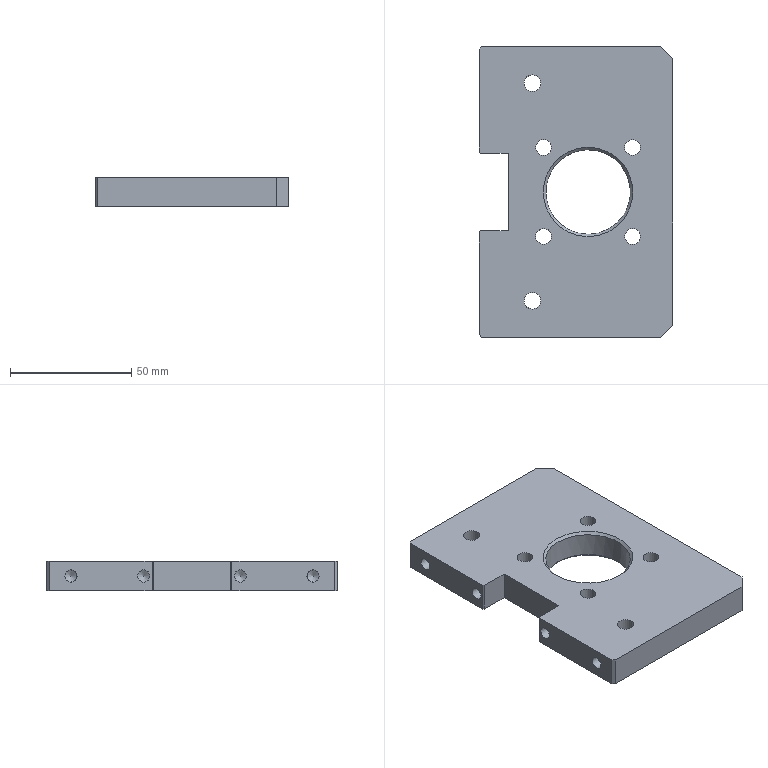Part | NX | 1 solid | 33 faces | box 80 x 120 x 12 mm | volume 94547 mm3 | plane 16 | cylinder 11 | cone 6 | commonest cylinder face diameters 5 x4 6.5 x4 6.8 x2 35 x1
STEP:
#1=CARTESIAN_POINT('',(-18.,41.6,0.));
#2=VERTEX_POINT('',#1);
#3=CARTESIAN_POINT('',(-18.,45.,0.));
#4=DIRECTION('',(0.,0.,1.));
#5=DIRECTION('',(0.,-1.,0.));
#6=AXIS2_PLACEMENT_3D('',#3,#4,#5);
#7=CIRCLE('',#6,3.4);
#8=EDGE_CURVE('',#2,#2,#7,.T.);
#9=ORIENTED_EDGE('',*,*,#8,.F.);
#10=EDGE_LOOP('',(#9));
#11=FACE_BOUND('',#10,.T.);
#12=CARTESIAN_POINT('',(5.,18.5,0.));
#13=VERTEX_POINT('',#12);
#14=CARTESIAN_POINT('',(5.,0.,0.));
#15=DIRECTION('',(0.,0.,-1.));
#16=DIRECTION('',(0.,1.,0.));
#17=AXIS2_PLACEMENT_3D('',#14,#15,#16);
#18=CIRCLE('',#17,18.5);
#19=EDGE_CURVE('',#13,#13,#18,.T.);
#20=ORIENTED_EDGE('',*,*,#19,.T.);
#21=EDGE_LOOP('',(#20));
#22=FACE_BOUND('',#21,.T.);
#23=CARTESIAN_POINT('',(23.385,-15.135,0.));
#24=VERTEX_POINT('',#23);
#25=CARTESIAN_POINT('',(23.385,-18.385,0.));
#26=DIRECTION('',(0.,0.,1.));
#27=DIRECTION('',(0.,1.,0.));
#28=AXIS2_PLACEMENT_3D('',#25,#26,#27);
#29=CIRCLE('',#28,3.25);
#30=EDGE_CURVE('',#24,#24,#29,.T.);
#31=ORIENTED_EDGE('',*,*,#30,.F.);
#32=EDGE_LOOP('',(#31));
#33=FACE_BOUND('',#32,.T.);
#34=CARTESIAN_POINT('',(-10.135,-18.385,0.));
#35=VERTEX_POINT('',#34);
#36=CARTESIAN_POINT('',(-13.385,-18.385,0.));
#37=DIRECTION('',(0.,0.,1.));
#38=DIRECTION('',(1.,0.,0.));
#39=AXIS2_PLACEMENT_3D('',#36,#37,#38);
#40=CIRCLE('',#39,3.25);
#41=EDGE_CURVE('',#35,#35,#40,.T.);
#42=ORIENTED_EDGE('',*,*,#41,.F.);
#43=EDGE_LOOP('',(#42));
#44=FACE_BOUND('',#43,.T.);
#45=CARTESIAN_POINT('',(-13.385,15.135,0.));
#46=VERTEX_POINT('',#45);
#47=CARTESIAN_POINT('',(-13.385,18.385,0.));
#48=DIRECTION('',(0.,0.,1.));
#49=DIRECTION('',(0.,-1.,0.));
#50=AXIS2_PLACEMENT_3D('',#47,#48,#49);
#51=CIRCLE('',#50,3.25);
#52=EDGE_CURVE('',#46,#46,#51,.T.);
#53=ORIENTED_EDGE('',*,*,#52,.F.);
#54=EDGE_LOOP('',(#53));
#55=FACE_BOUND('',#54,.T.);
#56=CARTESIAN_POINT('',(20.135,18.385,0.));
#57=VERTEX_POINT('',#56);
#58=CARTESIAN_POINT('',(23.385,18.385,0.));
#59=DIRECTION('',(0.,0.,1.));
#60=DIRECTION('',(-1.,0.,0.));
#61=AXIS2_PLACEMENT_3D('',#58,#59,#60);
#62=CIRCLE('',#61,3.25);
#63=EDGE_CURVE('',#57,#57,#62,.T.);
#64=ORIENTED_EDGE('',*,*,#63,.F.);
#65=EDGE_LOOP('',(#64));
#66=FACE_BOUND('',#65,.T.);
#67=CARTESIAN_POINT('',(-39.5,-16.,0.));
#68=VERTEX_POINT('',#67);
#69=CARTESIAN_POINT('',(-28.,-16.,0.));
#70=VERTEX_POINT('',#69);
#71=CARTESIAN_POINT('',(-52.,-16.,0.));
#72=DIRECTION('',(1.,0.,0.));
#73=VECTOR('',#72,1000.);
#74=LINE('',#71,#73);
#75=EDGE_CURVE('',#68,#70,#74,.T.);
#76=ORIENTED_EDGE('',*,*,#75,.F.);
#77=CARTESIAN_POINT('',(-40.,-16.5,0.));
#78=VERTEX_POINT('',#77);
#79=CARTESIAN_POINT('',(-40.,-16.5,0.));
#80=DIRECTION('',(0.7071,0.7071,0.));
#81=VECTOR('',#80,1000.);
#82=LINE('',#79,#81);
#83=EDGE_CURVE('',#68,#78,#82,.F.);
#84=ORIENTED_EDGE('',*,*,#83,.T.);
#85=CARTESIAN_POINT('',(-40.,-59.,0.));
#86=VERTEX_POINT('',#85);
#87=CARTESIAN_POINT('',(-40.,-60.,0.));
#88=DIRECTION('',(0.,1.,0.));
#89=VECTOR('',#88,1000.);
#90=LINE('',#87,#89);
#91=EDGE_CURVE('',#86,#78,#90,.T.);
#92=ORIENTED_EDGE('',*,*,#91,.F.);
#93=CARTESIAN_POINT('',(-39.,-60.,0.));
#94=VERTEX_POINT('',#93);
#95=CARTESIAN_POINT('',(-39.,-60.,0.));
#96=DIRECTION('',(-0.7071,0.7071,0.));
#97=VECTOR('',#96,1000.);
#98=LINE('',#95,#97);
#99=EDGE_CURVE('',#86,#94,#98,.F.);
#100=ORIENTED_EDGE('',*,*,#99,.T.);
#101=CARTESIAN_POINT('',(35.,-60.,0.));
#102=VERTEX_POINT('',#101);
#103=CARTESIAN_POINT('',(-40.,-60.,0.));
#104=DIRECTION('',(-1.,0.,0.));
#105=VECTOR('',#104,1000.);
#106=LINE('',#103,#105);
#107=EDGE_CURVE('',#102,#94,#106,.T.);
#108=ORIENTED_EDGE('',*,*,#107,.F.);
#109=CARTESIAN_POINT('',(40.,-55.,0.));
#110=VERTEX_POINT('',#109);
#111=CARTESIAN_POINT('',(40.,-55.,0.));
#112=DIRECTION('',(-0.7071,-0.7071,0.));
#113=VECTOR('',#112,1000.);
#114=LINE('',#111,#113);
#115=EDGE_CURVE('',#110,#102,#114,.T.);
#116=ORIENTED_EDGE('',*,*,#115,.F.);
#117=CARTESIAN_POINT('',(40.,55.,0.));
#118=VERTEX_POINT('',#117);
#119=CARTESIAN_POINT('',(40.,-60.,0.));
#120=DIRECTION('',(0.,1.,0.));
#121=VECTOR('',#120,1000.);
#122=LINE('',#119,#121);
#123=EDGE_CURVE('',#110,#118,#122,.T.);
#124=ORIENTED_EDGE('',*,*,#123,.T.);
#125=CARTESIAN_POINT('',(35.,60.,0.));
#126=VERTEX_POINT('',#125);
#127=CARTESIAN_POINT('',(40.,55.,0.));
#128=DIRECTION('',(0.7071,-0.7071,0.));
#129=VECTOR('',#128,1000.);
#130=LINE('',#127,#129);
#131=EDGE_CURVE('',#126,#118,#130,.T.);
#132=ORIENTED_EDGE('',*,*,#131,.F.);
#133=CARTESIAN_POINT('',(-39.,60.,0.));
#134=VERTEX_POINT('',#133);
#135=CARTESIAN_POINT('',(-40.,60.,0.));
#136=DIRECTION('',(-1.,0.,0.));
#137=VECTOR('',#136,1000.);
#138=LINE('',#135,#137);
#139=EDGE_CURVE('',#126,#134,#138,.T.);
#140=ORIENTED_EDGE('',*,*,#139,.T.);
#141=CARTESIAN_POINT('',(-40.,59.,0.));
#142=VERTEX_POINT('',#141);
#143=CARTESIAN_POINT('',(-40.,59.,0.));
#144=DIRECTION('',(-0.7071,-0.7071,0.));
#145=VECTOR('',#144,1000.);
#146=LINE('',#143,#145);
#147=EDGE_CURVE('',#134,#142,#146,.T.);
#148=ORIENTED_EDGE('',*,*,#147,.T.);
#149=CARTESIAN_POINT('',(-40.,16.5,0.));
#150=VERTEX_POINT('',#149);
#151=CARTESIAN_POINT('',(-40.,-60.,0.));
#152=DIRECTION('',(0.,1.,0.));
#153=VECTOR('',#152,1000.);
#154=LINE('',#151,#153);
#155=EDGE_CURVE('',#150,#142,#154,.T.);
#156=ORIENTED_EDGE('',*,*,#155,.F.);
#157=CARTESIAN_POINT('',(-39.5,16.,0.));
#158=VERTEX_POINT('',#157);
#159=CARTESIAN_POINT('',(-40.,16.5,0.));
#160=DIRECTION('',(-0.7071,0.7071,0.));
#161=VECTOR('',#160,1000.);
#162=LINE('',#159,#161);
#163=EDGE_CURVE('',#150,#158,#162,.F.);
#164=ORIENTED_EDGE('',*,*,#163,.T.);
#165=CARTESIAN_POINT('',(-28.,16.,0.));
#166=VERTEX_POINT('',#165);
#167=CARTESIAN_POINT('',(-52.,16.,0.));
#168=DIRECTION('',(-1.,0.,0.));
#169=VECTOR('',#168,1000.);
#170=LINE('',#167,#169);
#171=EDGE_CURVE('',#166,#158,#170,.T.);
#172=ORIENTED_EDGE('',*,*,#171,.F.);
#173=CARTESIAN_POINT('',(-28.,-16.,0.));
#174=DIRECTION('',(0.,1.,0.));
#175=VECTOR('',#174,1000.);
#176=LINE('',#173,#175);
#177=EDGE_CURVE('',#70,#166,#176,.T.);
#178=ORIENTED_EDGE('',*,*,#177,.F.);
#179=EDGE_LOOP('',(#76,#84,#92,#100,#108,#116,#124,#132,#140,#148,#156,#164,#172,#178));
#180=FACE_BOUND('',#179,.T.);
#181=CARTESIAN_POINT('',(-18.,-48.4,0.));
#182=VERTEX_POINT('',#181);
#183=CARTESIAN_POINT('',(-18.,-45.,0.));
#184=DIRECTION('',(0.,0.,1.));
#185=DIRECTION('',(0.,-1.,0.));
#186=AXIS2_PLACEMENT_3D('',#183,#184,#185);
#187=CIRCLE('',#186,3.4);
#188=EDGE_CURVE('',#182,#182,#187,.T.);
#189=ORIENTED_EDGE('',*,*,#188,.F.);
#190=EDGE_LOOP('',(#189));
#191=FACE_BOUND('',#190,.T.);
#192=CARTESIAN_POINT('',(-40.,-60.,0.));
#193=DIRECTION('',(0.,0.,-1.));
#194=DIRECTION('',(0.,1.,0.));
#195=AXIS2_PLACEMENT_3D('',#192,#193,#194);
#196=PLANE('',#195);
#197=ADVANCED_FACE('',(#11,#22,#33,#44,#55,#66,#180,#191),#196,.F.);
#198=CARTESIAN_POINT('',(-40.,-52.5,-6.));
#199=VERTEX_POINT('',#198);
#200=CARTESIAN_POINT('',(-40.,-50.,-6.));
#201=DIRECTION('',(-1.,0.,0.));
#202=DIRECTION('',(0.,-1.,0.));
#203=AXIS2_PLACEMENT_3D('',#200,#201,#202);
#204=CIRCLE('',#203,2.5);
#205=EDGE_CURVE('',#199,#199,#204,.T.);
#206=ORIENTED_EDGE('',*,*,#205,.F.);
#207=EDGE_LOOP('',(#206));
#208=FACE_BOUND('',#207,.T.);
#209=CARTESIAN_POINT('',(-40.,-22.5,-6.));
#210=VERTEX_POINT('',#209);
#211=CARTESIAN_POINT('',(-40.,-20.,-6.));
#212=DIRECTION('',(-1.,0.,0.));
#213=DIRECTION('',(0.,-1.,0.));
#214=AXIS2_PLACEMENT_3D('',#211,#212,#213);
#215=CIRCLE('',#214,2.5);
#216=EDGE_CURVE('',#210,#210,#215,.T.);
#217=ORIENTED_EDGE('',*,*,#216,.F.);
#218=EDGE_LOOP('',(#217));
#219=FACE_BOUND('',#218,.T.);
#220=ORIENTED_EDGE('',*,*,#91,.T.);
#221=CARTESIAN_POINT('',(-40.,-16.5,-12.));
#222=VERTEX_POINT('',#221);
#223=CARTESIAN_POINT('',(-40.,-16.5,-12.));
#224=DIRECTION('',(0.,0.,-1.));
#225=VECTOR('',#224,1000.);
#226=LINE('',#223,#225);
#227=EDGE_CURVE('',#78,#222,#226,.T.);
#228=ORIENTED_EDGE('',*,*,#227,.T.);
#229=CARTESIAN_POINT('',(-40.,-59.,-12.));
#230=VERTEX_POINT('',#229);
#231=CARTESIAN_POINT('',(-40.,-60.,-12.));
#232=DIRECTION('',(0.,1.,0.));
#233=VECTOR('',#232,1000.);
#234=LINE('',#231,#233);
#235=EDGE_CURVE('',#230,#222,#234,.T.);
#236=ORIENTED_EDGE('',*,*,#235,.F.);
#237=CARTESIAN_POINT('',(-40.,-59.,-12.));
#238=DIRECTION('',(0.,0.,1.));
#239=VECTOR('',#238,1000.);
#240=LINE('',#237,#239);
#241=EDGE_CURVE('',#230,#86,#240,.T.);
#242=ORIENTED_EDGE('',*,*,#241,.T.);
#243=EDGE_LOOP('',(#220,#228,#236,#242));
#244=FACE_BOUND('',#243,.T.);
#245=CARTESIAN_POINT('',(-40.,-60.,-12.));
#246=DIRECTION('',(1.,0.,0.));
#247=DIRECTION('',(0.,1.,0.));
#248=AXIS2_PLACEMENT_3D('',#245,#246,#247);
#249=PLANE('',#248);
#250=ADVANCED_FACE('',(#208,#219,#244),#249,.F.);
#251=CARTESIAN_POINT('',(-18.,41.6,-12.));
#252=VERTEX_POINT('',#251);
#253=CARTESIAN_POINT('',(-18.,45.,-12.));
#254=DIRECTION('',(0.,0.,1.));
#255=DIRECTION('',(0.,-1.,0.));
#256=AXIS2_PLACEMENT_3D('',#253,#254,#255);
#257=CIRCLE('',#256,3.4);
#258=EDGE_CURVE('',#252,#252,#257,.T.);
#259=ORIENTED_EDGE('',*,*,#258,.T.);
#260=EDGE_LOOP('',(#259));
#261=FACE_BOUND('',#260,.T.);
#262=CARTESIAN_POINT('',(-18.,-48.4,-12.));
#263=VERTEX_POINT('',#262);
#264=CARTESIAN_POINT('',(-18.,-45.,-12.));
#265=DIRECTION('',(0.,0.,1.));
#266=DIRECTION('',(0.,-1.,0.));
#267=AXIS2_PLACEMENT_3D('',#264,#265,#266);
#268=CIRCLE('',#267,3.4);
#269=EDGE_CURVE('',#263,#263,#268,.T.);
#270=ORIENTED_EDGE('',*,*,#269,.T.);
#271=EDGE_LOOP('',(#270));
#272=FACE_BOUND('',#271,.T.);
#273=CARTESIAN_POINT('',(-13.5,0.,-12.));
#274=VERTEX_POINT('',#273);
#275=CARTESIAN_POINT('',(5.,0.,-12.));
#276=DIRECTION('',(0.,0.,1.));
#277=DIRECTION('',(-1.,0.,0.));
#278=AXIS2_PLACEMENT_3D('',#275,#276,#277);
#279=CIRCLE('',#278,18.5);
#280=EDGE_CURVE('',#274,#274,#279,.T.);
#281=ORIENTED_EDGE('',*,*,#280,.T.);
#282=EDGE_LOOP('',(#281));
#283=FACE_BOUND('',#282,.T.);
#284=CARTESIAN_POINT('',(23.385,-15.135,-12.));
#285=VERTEX_POINT('',#284);
#286=CARTESIAN_POINT('',(23.385,-18.385,-12.));
#287=DIRECTION('',(0.,0.,1.));
#288=DIRECTION('',(0.,1.,0.));
#289=AXIS2_PLACEMENT_3D('',#286,#287,#288);
#290=CIRCLE('',#289,3.25);
#291=EDGE_CURVE('',#285,#285,#290,.T.);
#292=ORIENTED_EDGE('',*,*,#291,.T.);
#293=EDGE_LOOP('',(#292));
#294=FACE_BOUND('',#293,.T.);
#295=CARTESIAN_POINT('',(-10.135,-18.385,-12.));
#296=VERTEX_POINT('',#295);
#297=CARTESIAN_POINT('',(-13.385,-18.385,-12.));
#298=DIRECTION('',(0.,0.,1.));
#299=DIRECTION('',(1.,0.,0.));
#300=AXIS2_PLACEMENT_3D('',#297,#298,#299);
#301=CIRCLE('',#300,3.25);
#302=EDGE_CURVE('',#296,#296,#301,.T.);
#303=ORIENTED_EDGE('',*,*,#302,.T.);
#304=EDGE_LOOP('',(#303));
#305=FACE_BOUND('',#304,.T.);
#306=CARTESIAN_POINT('',(-13.385,15.135,-12.));
#307=VERTEX_POINT('',#306);
#308=CARTESIAN_POINT('',(-13.385,18.385,-12.));
#309=DIRECTION('',(0.,0.,1.));
#310=DIRECTION('',(0.,-1.,0.));
#311=AXIS2_PLACEMENT_3D('',#308,#309,#310);
#312=CIRCLE('',#311,3.25);
#313=EDGE_CURVE('',#307,#307,#312,.T.);
#314=ORIENTED_EDGE('',*,*,#313,.T.);
#315=EDGE_LOOP('',(#314));
#316=FACE_BOUND('',#315,.T.);
#317=CARTESIAN_POINT('',(20.135,18.385,-12.));
#318=VERTEX_POINT('',#317);
#319=CARTESIAN_POINT('',(23.385,18.385,-12.));
#320=DIRECTION('',(0.,0.,1.));
#321=DIRECTION('',(-1.,0.,0.));
#322=AXIS2_PLACEMENT_3D('',#319,#320,#321);
#323=CIRCLE('',#322,3.25);
#324=EDGE_CURVE('',#318,#318,#323,.T.);
#325=ORIENTED_EDGE('',*,*,#324,.T.);
#326=EDGE_LOOP('',(#325));
#327=FACE_BOUND('',#326,.T.);
#328=ORIENTED_EDGE('',*,*,#235,.T.);
#329=CARTESIAN_POINT('',(-39.5,-16.,-12.));
#330=VERTEX_POINT('',#329);
#331=CARTESIAN_POINT('',(-40.,-16.5,-12.));
#332=DIRECTION('',(-0.7071,-0.7071,0.));
#333=VECTOR('',#332,1000.);
#334=LINE('',#331,#333);
#335=EDGE_CURVE('',#222,#330,#334,.F.);
#336=ORIENTED_EDGE('',*,*,#335,.T.);
#337=CARTESIAN_POINT('',(-28.,-16.,-12.));
#338=VERTEX_POINT('',#337);
#339=CARTESIAN_POINT('',(-52.,-16.,-12.));
#340=DIRECTION('',(1.,0.,0.));
#341=VECTOR('',#340,1000.);
#342=LINE('',#339,#341);
#343=EDGE_CURVE('',#330,#338,#342,.T.);
#344=ORIENTED_EDGE('',*,*,#343,.T.);
#345=CARTESIAN_POINT('',(-28.,16.,-12.));
#346=VERTEX_POINT('',#345);
#347=CARTESIAN_POINT('',(-28.,-16.,-12.));
#348=DIRECTION('',(0.,1.,0.));
#349=VECTOR('',#348,1000.);
#350=LINE('',#347,#349);
#351=EDGE_CURVE('',#338,#346,#350,.T.);
#352=ORIENTED_EDGE('',*,*,#351,.T.);
#353=CARTESIAN_POINT('',(-39.5,16.,-12.));
#354=VERTEX_POINT('',#353);
#355=CARTESIAN_POINT('',(-52.,16.,-12.));
#356=DIRECTION('',(-1.,0.,0.));
#357=VECTOR('',#356,1000.);
#358=LINE('',#355,#357);
#359=EDGE_CURVE('',#346,#354,#358,.T.);
#360=ORIENTED_EDGE('',*,*,#359,.T.);
#361=CARTESIAN_POINT('',(-40.,16.5,-12.));
#362=VERTEX_POINT('',#361);
#363=CARTESIAN_POINT('',(-40.,16.5,-12.));
#364=DIRECTION('',(0.7071,-0.7071,0.));
#365=VECTOR('',#364,1000.);
#366=LINE('',#363,#365);
#367=EDGE_CURVE('',#354,#362,#366,.F.);
#368=ORIENTED_EDGE('',*,*,#367,.T.);
#369=CARTESIAN_POINT('',(-40.,59.,-12.));
#370=VERTEX_POINT('',#369);
#371=CARTESIAN_POINT('',(-40.,-60.,-12.));
#372=DIRECTION('',(0.,1.,0.));
#373=VECTOR('',#372,1000.);
#374=LINE('',#371,#373);
#375=EDGE_CURVE('',#362,#370,#374,.T.);
#376=ORIENTED_EDGE('',*,*,#375,.T.);
#377=CARTESIAN_POINT('',(-39.,60.,-12.));
#378=VERTEX_POINT('',#377);
#379=CARTESIAN_POINT('',(-40.,59.,-12.));
#380=DIRECTION('',(0.7071,0.7071,0.));
#381=VECTOR('',#380,1000.);
#382=LINE('',#379,#381);
#383=EDGE_CURVE('',#370,#378,#382,.T.);
#384=ORIENTED_EDGE('',*,*,#383,.T.);
#385=CARTESIAN_POINT('',(35.,60.,-12.));
#386=VERTEX_POINT('',#385);
#387=CARTESIAN_POINT('',(40.,60.,-12.));
#388=DIRECTION('',(1.,0.,0.));
#389=VECTOR('',#388,1000.);
#390=LINE('',#387,#389);
#391=EDGE_CURVE('',#378,#386,#390,.T.);
#392=ORIENTED_EDGE('',*,*,#391,.T.);
#393=CARTESIAN_POINT('',(40.,55.,-12.));
#394=VERTEX_POINT('',#393);
#395=CARTESIAN_POINT('',(40.,55.,-12.));
#396=DIRECTION('',(0.7071,-0.7071,0.));
#397=VECTOR('',#396,1000.);
#398=LINE('',#395,#397);
#399=EDGE_CURVE('',#386,#394,#398,.T.);
#400=ORIENTED_EDGE('',*,*,#399,.T.);
#401=CARTESIAN_POINT('',(40.,-55.,-12.));
#402=VERTEX_POINT('',#401);
#403=CARTESIAN_POINT('',(40.,-60.,-12.));
#404=DIRECTION('',(0.,1.,0.));
#405=VECTOR('',#404,1000.);
#406=LINE('',#403,#405);
#407=EDGE_CURVE('',#402,#394,#406,.T.);
#408=ORIENTED_EDGE('',*,*,#407,.F.);
#409=CARTESIAN_POINT('',(35.,-60.,-12.));
#410=VERTEX_POINT('',#409);
#411=CARTESIAN_POINT('',(40.,-55.,-12.));
#412=DIRECTION('',(-0.7071,-0.7071,0.));
#413=VECTOR('',#412,1000.);
#414=LINE('',#411,#413);
#415=EDGE_CURVE('',#402,#410,#414,.T.);
#416=ORIENTED_EDGE('',*,*,#415,.T.);
#417=CARTESIAN_POINT('',(-39.,-60.,-12.));
#418=VERTEX_POINT('',#417);
#419=CARTESIAN_POINT('',(40.,-60.,-12.));
#420=DIRECTION('',(1.,0.,0.));
#421=VECTOR('',#420,1000.);
#422=LINE('',#419,#421);
#423=EDGE_CURVE('',#418,#410,#422,.T.);
#424=ORIENTED_EDGE('',*,*,#423,.F.);
#425=CARTESIAN_POINT('',(-39.,-60.,-12.));
#426=DIRECTION('',(0.7071,-0.7071,0.));
#427=VECTOR('',#426,1000.);
#428=LINE('',#425,#427);
#429=EDGE_CURVE('',#418,#230,#428,.F.);
#430=ORIENTED_EDGE('',*,*,#429,.T.);
#431=EDGE_LOOP('',(#328,#336,#344,#352,#360,#368,#376,#384,#392,#400,#408,#416,#424,#430));
#432=FACE_BOUND('',#431,.T.);
#433=CARTESIAN_POINT('',(40.,-60.,-12.));
#434=DIRECTION('',(0.,0.,1.));
#435=DIRECTION('',(-1.,0.,0.));
#436=AXIS2_PLACEMENT_3D('',#433,#434,#435);
#437=PLANE('',#436);
#438=ADVANCED_FACE('',(#261,#272,#283,#294,#305,#316,#327,#432),#437,.F.);
#439=ORIENTED_EDGE('',*,*,#123,.F.);
#440=CARTESIAN_POINT('',(40.,-55.,-12.));
#441=DIRECTION('',(0.,0.,1.));
#442=VECTOR('',#441,1000.);
#443=LINE('',#440,#442);
#444=EDGE_CURVE('',#402,#110,#443,.T.);
#445=ORIENTED_EDGE('',*,*,#444,.F.);
#446=ORIENTED_EDGE('',*,*,#407,.T.);
#447=CARTESIAN_POINT('',(40.,55.,-12.));
#448=DIRECTION('',(0.,0.,1.));
#449=VECTOR('',#448,1000.);
#450=LINE('',#447,#449);
#451=EDGE_CURVE('',#394,#118,#450,.T.);
#452=ORIENTED_EDGE('',*,*,#451,.T.);
#453=EDGE_LOOP('',(#439,#445,#446,#452));
#454=FACE_BOUND('',#453,.T.);
#455=CARTESIAN_POINT('',(40.,-60.,0.));
#456=DIRECTION('',(-1.,0.,0.));
#457=DIRECTION('',(0.,0.,-1.));
#458=AXIS2_PLACEMENT_3D('',#455,#456,#457);
#459=PLANE('',#458);
#460=ADVANCED_FACE('',(#454),#459,.F.);
#461=CARTESIAN_POINT('',(-40.,47.5,-6.));
#462=VERTEX_POINT('',#461);
#463=CARTESIAN_POINT('',(-40.,50.,-6.));
#464=DIRECTION('',(-1.,0.,0.));
#465=DIRECTION('',(0.,-1.,0.));
#466=AXIS2_PLACEMENT_3D('',#463,#464,#465);
#467=CIRCLE('',#466,2.5);
#468=EDGE_CURVE('',#462,#462,#467,.T.);
#469=ORIENTED_EDGE('',*,*,#468,.F.);
#470=EDGE_LOOP('',(#469));
#471=FACE_BOUND('',#470,.T.);
#472=CARTESIAN_POINT('',(-40.,17.5,-6.));
#473=VERTEX_POINT('',#472);
#474=CARTESIAN_POINT('',(-40.,20.,-6.));
#475=DIRECTION('',(-1.,0.,0.));
#476=DIRECTION('',(0.,-1.,0.));
#477=AXIS2_PLACEMENT_3D('',#474,#475,#476);
#478=CIRCLE('',#477,2.5);
#479=EDGE_CURVE('',#473,#473,#478,.T.);
#480=ORIENTED_EDGE('',*,*,#479,.F.);
#481=EDGE_LOOP('',(#480));
#482=FACE_BOUND('',#481,.T.);
#483=ORIENTED_EDGE('',*,*,#375,.F.);
#484=CARTESIAN_POINT('',(-40.,16.5,-12.));
#485=DIRECTION('',(0.,0.,1.));
#486=VECTOR('',#485,1000.);
#487=LINE('',#484,#486);
#488=EDGE_CURVE('',#362,#150,#487,.T.);
#489=ORIENTED_EDGE('',*,*,#488,.T.);
#490=ORIENTED_EDGE('',*,*,#155,.T.);
#491=CARTESIAN_POINT('',(-40.,59.,-12.));
#492=DIRECTION('',(0.,0.,-1.));
#493=VECTOR('',#492,1000.);
#494=LINE('',#491,#493);
#495=EDGE_CURVE('',#142,#370,#494,.T.);
#496=ORIENTED_EDGE('',*,*,#495,.T.);
#497=EDGE_LOOP('',(#483,#489,#490,#496));
#498=FACE_BOUND('',#497,.T.);
#499=CARTESIAN_POINT('',(-40.,-60.,-12.));
#500=DIRECTION('',(1.,0.,0.));
#501=DIRECTION('',(0.,1.,0.));
#502=AXIS2_PLACEMENT_3D('',#499,#500,#501);
#503=PLANE('',#502);
#504=ADVANCED_FACE('',(#471,#482,#498),#503,.F.);
#505=ORIENTED_EDGE('',*,*,#107,.T.);
#506=CARTESIAN_POINT('',(-39.,-60.,-12.));
#507=DIRECTION('',(0.,0.,-1.));
#508=VECTOR('',#507,1000.);
#509=LINE('',#506,#508);
#510=EDGE_CURVE('',#94,#418,#509,.T.);
#511=ORIENTED_EDGE('',*,*,#510,.T.);
#512=ORIENTED_EDGE('',*,*,#423,.T.);
#513=CARTESIAN_POINT('',(35.,-60.,-12.));
#514=DIRECTION('',(0.,0.,1.));
#515=VECTOR('',#514,1000.);
#516=LINE('',#513,#515);
#517=EDGE_CURVE('',#410,#102,#516,.T.);
#518=ORIENTED_EDGE('',*,*,#517,.T.);
#519=EDGE_LOOP('',(#505,#511,#512,#518));
#520=FACE_BOUND('',#519,.T.);
#521=CARTESIAN_POINT('',(-40.,-60.,-12.));
#522=DIRECTION('',(0.,1.,0.));
#523=DIRECTION('',(-1.,0.,0.));
#524=AXIS2_PLACEMENT_3D('',#521,#522,#523);
#525=PLANE('',#524);
#526=ADVANCED_FACE('',(#520),#525,.F.);
#527=ORIENTED_EDGE('',*,*,#391,.F.);
#528=CARTESIAN_POINT('',(-39.,60.,0.));
#529=DIRECTION('',(0.,0.,1.));
#530=VECTOR('',#529,1000.);
#531=LINE('',#528,#530);
#532=EDGE_CURVE('',#378,#134,#531,.T.);
#533=ORIENTED_EDGE('',*,*,#532,.T.);
#534=ORIENTED_EDGE('',*,*,#139,.F.);
#535=CARTESIAN_POINT('',(35.,60.,-12.));
#536=DIRECTION('',(0.,0.,1.));
#537=VECTOR('',#536,1000.);
#538=LINE('',#535,#537);
#539=EDGE_CURVE('',#386,#126,#538,.T.);
#540=ORIENTED_EDGE('',*,*,#539,.F.);
#541=EDGE_LOOP('',(#527,#533,#534,#540));
#542=FACE_BOUND('',#541,.T.);
#543=CARTESIAN_POINT('',(-40.,60.,-12.));
#544=DIRECTION('',(0.,1.,0.));
#545=DIRECTION('',(-1.,0.,0.));
#546=AXIS2_PLACEMENT_3D('',#543,#544,#545);
#547=PLANE('',#546);
#548=ADVANCED_FACE('',(#542),#547,.T.);
#549=CARTESIAN_POINT('',(-18.557,-50.,-6.));
#550=VERTEX_POINT('',#549);
#551=VERTEX_LOOP('',#550);
#552=FACE_BOUND('',#551,.T.);
#553=CARTESIAN_POINT('',(-20.,-47.75,-7.089));
#554=VERTEX_POINT('',#553);
#555=CARTESIAN_POINT('',(-20.,-47.75,-4.911));
#556=VERTEX_POINT('',#555);
#557=CARTESIAN_POINT('',(-20.,-50.,-6.));
#558=DIRECTION('',(-1.,0.,0.));
#559=DIRECTION('',(0.,-1.,0.));
#560=AXIS2_PLACEMENT_3D('',#557,#558,#559);
#561=CIRCLE('',#560,2.5);
#562=EDGE_CURVE('',#554,#556,#561,.T.);
#563=ORIENTED_EDGE('',*,*,#562,.T.);
#564=CARTESIAN_POINT('',(-20.,-47.75,-4.911));
#565=CARTESIAN_POINT('',(-19.864,-47.848,-5.247));
#566=CARTESIAN_POINT('',(-19.669,-47.962,-5.995));
#567=CARTESIAN_POINT('',(-19.862,-47.85,-6.748));
#568=CARTESIAN_POINT('',(-20.,-47.75,-7.089));
#569=B_SPLINE_CURVE_WITH_KNOTS('',3,(#564,#565,#566,#567,#568),.UNSPECIFIED.,.F.,.F.,(4,1,4),(0.0003666,0.001491,0.002614),.UNSPECIFIED.);
#570=EDGE_CURVE('',#556,#554,#569,.T.);
#571=ORIENTED_EDGE('',*,*,#570,.T.);
#572=EDGE_LOOP('',(#563,#571));
#573=FACE_BOUND('',#572,.T.);
#574=CARTESIAN_POINT('',(-20.,-50.,-6.));
#575=DIRECTION('',(-1.,0.,0.));
#576=DIRECTION('',(0.,-1.,0.));
#577=AXIS2_PLACEMENT_3D('',#574,#575,#576);
#578=CONICAL_SURFACE('',#577,2.5,1.047);
#579=ADVANCED_FACE('',(#552,#573),#578,.F.);
#580=ORIENTED_EDGE('',*,*,#562,.F.);
#581=CARTESIAN_POINT('',(-20.,-47.75,-7.089));
#582=CARTESIAN_POINT('',(-20.204,-47.601,-6.782));
#583=CARTESIAN_POINT('',(-20.404,-47.399,-5.998));
#584=CARTESIAN_POINT('',(-20.204,-47.601,-5.218));
#585=CARTESIAN_POINT('',(-20.,-47.75,-4.911));
#586=B_SPLINE_CURVE_WITH_KNOTS('',3,(#581,#582,#583,#584,#585),.UNSPECIFIED.,.F.,.F.,(4,1,4),(0.,0.001176,0.002353),.UNSPECIFIED.);
#587=EDGE_CURVE('',#554,#556,#586,.T.);
#588=ORIENTED_EDGE('',*,*,#587,.T.);
#589=EDGE_LOOP('',(#580,#588));
#590=FACE_BOUND('',#589,.T.);
#591=ORIENTED_EDGE('',*,*,#205,.T.);
#592=EDGE_LOOP('',(#591));
#593=FACE_BOUND('',#592,.T.);
#594=CARTESIAN_POINT('',(-40.,-50.,-6.));
#595=DIRECTION('',(-1.,0.,0.));
#596=DIRECTION('',(0.,-1.,0.));
#597=AXIS2_PLACEMENT_3D('',#594,#595,#596);
#598=CYLINDRICAL_SURFACE('',#597,2.5);
#599=ADVANCED_FACE('',(#590,#593),#598,.F.);
#600=CARTESIAN_POINT('',(-18.557,-20.,-6.));
#601=VERTEX_POINT('',#600);
#602=VERTEX_LOOP('',#601);
#603=FACE_BOUND('',#602,.T.);
#604=CARTESIAN_POINT('',(-20.,-22.5,-6.));
#605=VERTEX_POINT('',#604);
#606=CARTESIAN_POINT('',(-20.,-20.,-6.));
#607=DIRECTION('',(-1.,0.,0.));
#608=DIRECTION('',(0.,-1.,0.));
#609=AXIS2_PLACEMENT_3D('',#606,#607,#608);
#610=CIRCLE('',#609,2.5);
#611=EDGE_CURVE('',#605,#605,#610,.T.);
#612=ORIENTED_EDGE('',*,*,#611,.T.);
#613=EDGE_LOOP('',(#612));
#614=FACE_BOUND('',#613,.T.);
#615=CARTESIAN_POINT('',(-20.,-20.,-6.));
#616=DIRECTION('',(-1.,0.,0.));
#617=DIRECTION('',(0.,-1.,0.));
#618=AXIS2_PLACEMENT_3D('',#615,#616,#617);
#619=CONICAL_SURFACE('',#618,2.5,1.047);
#620=ADVANCED_FACE('',(#603,#614),#619,.F.);
#621=ORIENTED_EDGE('',*,*,#611,.F.);
#622=EDGE_LOOP('',(#621));
#623=FACE_BOUND('',#622,.T.);
#624=ORIENTED_EDGE('',*,*,#216,.T.);
#625=EDGE_LOOP('',(#624));
#626=FACE_BOUND('',#625,.T.);
#627=CARTESIAN_POINT('',(-40.,-20.,-6.));
#628=DIRECTION('',(-1.,0.,0.));
#629=DIRECTION('',(0.,-1.,0.));
#630=AXIS2_PLACEMENT_3D('',#627,#628,#629);
#631=CYLINDRICAL_SURFACE('',#630,2.5);
#632=ADVANCED_FACE('',(#623,#626),#631,.F.);
#633=CARTESIAN_POINT('',(-18.557,20.,-6.));
#634=VERTEX_POINT('',#633);
#635=VERTEX_LOOP('',#634);
#636=FACE_BOUND('',#635,.T.);
#637=CARTESIAN_POINT('',(-20.,17.5,-6.));
#638=VERTEX_POINT('',#637);
#639=CARTESIAN_POINT('',(-20.,20.,-6.));
#640=DIRECTION('',(-1.,0.,0.));
#641=DIRECTION('',(0.,-1.,0.));
#642=AXIS2_PLACEMENT_3D('',#639,#640,#641);
#643=CIRCLE('',#642,2.5);
#644=EDGE_CURVE('',#638,#638,#643,.T.);
#645=ORIENTED_EDGE('',*,*,#644,.T.);
#646=EDGE_LOOP('',(#645));
#647=FACE_BOUND('',#646,.T.);
#648=CARTESIAN_POINT('',(-20.,20.,-6.));
#649=DIRECTION('',(-1.,0.,0.));
#650=DIRECTION('',(0.,-1.,0.));
#651=AXIS2_PLACEMENT_3D('',#648,#649,#650);
#652=CONICAL_SURFACE('',#651,2.5,1.047);
#653=ADVANCED_FACE('',(#636,#647),#652,.F.);
#654=ORIENTED_EDGE('',*,*,#644,.F.);
#655=EDGE_LOOP('',(#654));
#656=FACE_BOUND('',#655,.T.);
#657=ORIENTED_EDGE('',*,*,#479,.T.);
#658=EDGE_LOOP('',(#657));
#659=FACE_BOUND('',#658,.T.);
#660=CARTESIAN_POINT('',(-40.,20.,-6.));
#661=DIRECTION('',(-1.,0.,0.));
#662=DIRECTION('',(0.,-1.,0.));
#663=AXIS2_PLACEMENT_3D('',#660,#661,#662);
#664=CYLINDRICAL_SURFACE('',#663,2.5);
#665=ADVANCED_FACE('',(#656,#659),#664,.F.);
#666=CARTESIAN_POINT('',(-18.557,50.,-6.));
#667=VERTEX_POINT('',#666);
#668=VERTEX_LOOP('',#667);
#669=FACE_BOUND('',#668,.T.);
#670=CARTESIAN_POINT('',(-20.,47.75,-4.911));
#671=VERTEX_POINT('',#670);
#672=CARTESIAN_POINT('',(-20.,47.75,-7.089));
#673=VERTEX_POINT('',#672);
#674=CARTESIAN_POINT('',(-20.,50.,-6.));
#675=DIRECTION('',(-1.,0.,0.));
#676=DIRECTION('',(0.,-1.,0.));
#677=AXIS2_PLACEMENT_3D('',#674,#675,#676);
#678=CIRCLE('',#677,2.5);
#679=EDGE_CURVE('',#671,#673,#678,.T.);
#680=ORIENTED_EDGE('',*,*,#679,.T.);
#681=CARTESIAN_POINT('',(-20.,47.75,-7.089));
#682=CARTESIAN_POINT('',(-19.864,47.848,-6.753));
#683=CARTESIAN_POINT('',(-19.669,47.962,-6.005));
#684=CARTESIAN_POINT('',(-19.862,47.85,-5.252));
#685=CARTESIAN_POINT('',(-20.,47.75,-4.911));
#686=B_SPLINE_CURVE_WITH_KNOTS('',3,(#681,#682,#683,#684,#685),.UNSPECIFIED.,.F.,.F.,(4,1,4),(0.0003666,0.001491,0.002614),.UNSPECIFIED.);
#687=EDGE_CURVE('',#673,#671,#686,.T.);
#688=ORIENTED_EDGE('',*,*,#687,.T.);
#689=EDGE_LOOP('',(#680,#688));
#690=FACE_BOUND('',#689,.T.);
#691=CARTESIAN_POINT('',(-20.,50.,-6.));
#692=DIRECTION('',(-1.,0.,0.));
#693=DIRECTION('',(0.,-1.,0.));
#694=AXIS2_PLACEMENT_3D('',#691,#692,#693);
#695=CONICAL_SURFACE('',#694,2.5,1.047);
#696=ADVANCED_FACE('',(#669,#690),#695,.F.);
#697=ORIENTED_EDGE('',*,*,#679,.F.);
#698=CARTESIAN_POINT('',(-20.,47.75,-4.911));
#699=CARTESIAN_POINT('',(-20.204,47.601,-5.218));
#700=CARTESIAN_POINT('',(-20.404,47.399,-6.002));
#701=CARTESIAN_POINT('',(-20.204,47.601,-6.782));
#702=CARTESIAN_POINT('',(-20.,47.75,-7.089));
#703=B_SPLINE_CURVE_WITH_KNOTS('',3,(#698,#699,#700,#701,#702),.UNSPECIFIED.,.F.,.F.,(4,1,4),(0.,0.001176,0.002353),.UNSPECIFIED.);
#704=EDGE_CURVE('',#671,#673,#703,.T.);
#705=ORIENTED_EDGE('',*,*,#704,.T.);
#706=EDGE_LOOP('',(#697,#705));
#707=FACE_BOUND('',#706,.T.);
#708=ORIENTED_EDGE('',*,*,#468,.T.);
#709=EDGE_LOOP('',(#708));
#710=FACE_BOUND('',#709,.T.);
#711=CARTESIAN_POINT('',(-40.,50.,-6.));
#712=DIRECTION('',(-1.,0.,0.));
#713=DIRECTION('',(0.,-1.,0.));
#714=AXIS2_PLACEMENT_3D('',#711,#712,#713);
#715=CYLINDRICAL_SURFACE('',#714,2.5);
#716=ADVANCED_FACE('',(#707,#710),#715,.F.);
#717=CARTESIAN_POINT('',(5.,17.5,-1.));
#718=VERTEX_POINT('',#717);
#719=CARTESIAN_POINT('',(5.,0.,-1.));
#720=DIRECTION('',(0.,0.,-1.));
#721=DIRECTION('',(0.,1.,0.));
#722=AXIS2_PLACEMENT_3D('',#719,#720,#721);
#723=CIRCLE('',#722,17.5);
#724=EDGE_CURVE('',#718,#718,#723,.F.);
#725=ORIENTED_EDGE('',*,*,#724,.T.);
#726=EDGE_LOOP('',(#725));
#727=FACE_BOUND('',#726,.T.);
#728=CARTESIAN_POINT('',(5.,-17.5,-11.));
#729=VERTEX_POINT('',#728);
#730=CARTESIAN_POINT('',(5.,0.,-11.));
#731=DIRECTION('',(0.,0.,1.));
#732=DIRECTION('',(0.,-1.,0.));
#733=AXIS2_PLACEMENT_3D('',#730,#731,#732);
#734=CIRCLE('',#733,17.5);
#735=EDGE_CURVE('',#729,#729,#734,.F.);
#736=ORIENTED_EDGE('',*,*,#735,.T.);
#737=EDGE_LOOP('',(#736));
#738=FACE_BOUND('',#737,.T.);
#739=CARTESIAN_POINT('',(5.,0.,-12.));
#740=DIRECTION('',(0.,0.,1.));
#741=DIRECTION('',(0.,-1.,0.));
#742=AXIS2_PLACEMENT_3D('',#739,#740,#741);
#743=CYLINDRICAL_SURFACE('',#742,17.5);
#744=ADVANCED_FACE('',(#727,#738),#743,.F.);
#745=ORIENTED_EDGE('',*,*,#324,.F.);
#746=EDGE_LOOP('',(#745));
#747=FACE_BOUND('',#746,.T.);
#748=ORIENTED_EDGE('',*,*,#63,.T.);
#749=EDGE_LOOP('',(#748));
#750=FACE_BOUND('',#749,.T.);
#751=CARTESIAN_POINT('',(23.385,18.385,-12.));
#752=DIRECTION('',(0.,0.,1.));
#753=DIRECTION('',(-1.,0.,0.));
#754=AXIS2_PLACEMENT_3D('',#751,#752,#753);
#755=CYLINDRICAL_SURFACE('',#754,3.25);
#756=ADVANCED_FACE('',(#747,#750),#755,.F.);
#757=ORIENTED_EDGE('',*,*,#313,.F.);
#758=EDGE_LOOP('',(#757));
#759=FACE_BOUND('',#758,.T.);
#760=ORIENTED_EDGE('',*,*,#52,.T.);
#761=EDGE_LOOP('',(#760));
#762=FACE_BOUND('',#761,.T.);
#763=CARTESIAN_POINT('',(-13.385,18.385,-12.));
#764=DIRECTION('',(0.,0.,1.));
#765=DIRECTION('',(0.,-1.,0.));
#766=AXIS2_PLACEMENT_3D('',#763,#764,#765);
#767=CYLINDRICAL_SURFACE('',#766,3.25);
#768=ADVANCED_FACE('',(#759,#762),#767,.F.);
#769=ORIENTED_EDGE('',*,*,#302,.F.);
#770=EDGE_LOOP('',(#769));
#771=FACE_BOUND('',#770,.T.);
#772=ORIENTED_EDGE('',*,*,#41,.T.);
#773=EDGE_LOOP('',(#772));
#774=FACE_BOUND('',#773,.T.);
#775=CARTESIAN_POINT('',(-13.385,-18.385,-12.));
#776=DIRECTION('',(0.,0.,1.));
#777=DIRECTION('',(1.,0.,0.));
#778=AXIS2_PLACEMENT_3D('',#775,#776,#777);
#779=CYLINDRICAL_SURFACE('',#778,3.25);
#780=ADVANCED_FACE('',(#771,#774),#779,.F.);
#781=ORIENTED_EDGE('',*,*,#291,.F.);
#782=EDGE_LOOP('',(#781));
#783=FACE_BOUND('',#782,.T.);
#784=ORIENTED_EDGE('',*,*,#30,.T.);
#785=EDGE_LOOP('',(#784));
#786=FACE_BOUND('',#785,.T.);
#787=CARTESIAN_POINT('',(23.385,-18.385,-12.));
#788=DIRECTION('',(0.,0.,1.));
#789=DIRECTION('',(0.,1.,0.));
#790=AXIS2_PLACEMENT_3D('',#787,#788,#789);
#791=CYLINDRICAL_SURFACE('',#790,3.25);
#792=ADVANCED_FACE('',(#783,#786),#791,.F.);
#793=ORIENTED_EDGE('',*,*,#19,.F.);
#794=EDGE_LOOP('',(#793));
#795=FACE_BOUND('',#794,.T.);
#796=ORIENTED_EDGE('',*,*,#724,.F.);
#797=EDGE_LOOP('',(#796));
#798=FACE_BOUND('',#797,.T.);
#799=CARTESIAN_POINT('',(5.,0.,-1.));
#800=DIRECTION('',(0.,0.,1.));
#801=DIRECTION('',(0.,-1.,0.));
#802=AXIS2_PLACEMENT_3D('',#799,#800,#801);
#803=CONICAL_SURFACE('',#802,17.5,0.7854);
#804=ADVANCED_FACE('',(#795,#798),#803,.F.);
#805=ORIENTED_EDGE('',*,*,#735,.F.);
#806=EDGE_LOOP('',(#805));
#807=FACE_BOUND('',#806,.T.);
#808=ORIENTED_EDGE('',*,*,#280,.F.);
#809=EDGE_LOOP('',(#808));
#810=FACE_BOUND('',#809,.T.);
#811=CARTESIAN_POINT('',(5.,0.,-12.));
#812=DIRECTION('',(0.,0.,-1.));
#813=DIRECTION('',(0.,1.,0.));
#814=AXIS2_PLACEMENT_3D('',#811,#812,#813);
#815=CONICAL_SURFACE('',#814,18.5,0.7854);
#816=ADVANCED_FACE('',(#807,#810),#815,.F.);
#817=ORIENTED_EDGE('',*,*,#131,.T.);
#818=ORIENTED_EDGE('',*,*,#451,.F.);
#819=ORIENTED_EDGE('',*,*,#399,.F.);
#820=ORIENTED_EDGE('',*,*,#539,.T.);
#821=EDGE_LOOP('',(#817,#818,#819,#820));
#822=FACE_BOUND('',#821,.T.);
#823=CARTESIAN_POINT('',(40.,55.,-12.));
#824=DIRECTION('',(-0.7071,-0.7071,0.));
#825=DIRECTION('',(0.7071,-0.7071,0.));
#826=AXIS2_PLACEMENT_3D('',#823,#824,#825);
#827=PLANE('',#826);
#828=ADVANCED_FACE('',(#822),#827,.F.);
#829=ORIENTED_EDGE('',*,*,#115,.T.);
#830=ORIENTED_EDGE('',*,*,#517,.F.);
#831=ORIENTED_EDGE('',*,*,#415,.F.);
#832=ORIENTED_EDGE('',*,*,#444,.T.);
#833=EDGE_LOOP('',(#829,#830,#831,#832));
#834=FACE_BOUND('',#833,.T.);
#835=CARTESIAN_POINT('',(40.,-55.,-12.));
#836=DIRECTION('',(-0.7071,0.7071,0.));
#837=DIRECTION('',(-0.7071,-0.7071,0.));
#838=AXIS2_PLACEMENT_3D('',#835,#836,#837);
#839=PLANE('',#838);
#840=ADVANCED_FACE('',(#834),#839,.F.);
#841=ORIENTED_EDGE('',*,*,#99,.F.);
#842=ORIENTED_EDGE('',*,*,#241,.F.);
#843=ORIENTED_EDGE('',*,*,#429,.F.);
#844=ORIENTED_EDGE('',*,*,#510,.F.);
#845=EDGE_LOOP('',(#841,#842,#843,#844));
#846=FACE_BOUND('',#845,.T.);
#847=CARTESIAN_POINT('',(-39.,-60.,-12.));
#848=DIRECTION('',(0.7071,0.7071,0.));
#849=DIRECTION('',(0.,0.,-1.));
#850=AXIS2_PLACEMENT_3D('',#847,#848,#849);
#851=PLANE('',#850);
#852=ADVANCED_FACE('',(#846),#851,.F.);
#853=ORIENTED_EDGE('',*,*,#147,.F.);
#854=ORIENTED_EDGE('',*,*,#532,.F.);
#855=ORIENTED_EDGE('',*,*,#383,.F.);
#856=ORIENTED_EDGE('',*,*,#495,.F.);
#857=EDGE_LOOP('',(#853,#854,#855,#856));
#858=FACE_BOUND('',#857,.T.);
#859=CARTESIAN_POINT('',(-40.,59.,-12.));
#860=DIRECTION('',(-0.7071,0.7071,0.));
#861=DIRECTION('',(0.,0.,1.));
#862=AXIS2_PLACEMENT_3D('',#859,#860,#861);
#863=PLANE('',#862);
#864=ADVANCED_FACE('',(#858),#863,.T.);
#865=ORIENTED_EDGE('',*,*,#343,.F.);
#866=CARTESIAN_POINT('',(-39.5,-16.,-12.));
#867=DIRECTION('',(0.,0.,1.));
#868=VECTOR('',#867,1000.);
#869=LINE('',#866,#868);
#870=EDGE_CURVE('',#330,#68,#869,.T.);
#871=ORIENTED_EDGE('',*,*,#870,.T.);
#872=ORIENTED_EDGE('',*,*,#75,.T.);
#873=CARTESIAN_POINT('',(-28.,-16.,-12.));
#874=DIRECTION('',(0.,0.,1.));
#875=VECTOR('',#874,1000.);
#876=LINE('',#873,#875);
#877=EDGE_CURVE('',#338,#70,#876,.T.);
#878=ORIENTED_EDGE('',*,*,#877,.F.);
#879=EDGE_LOOP('',(#865,#871,#872,#878));
#880=FACE_BOUND('',#879,.T.);
#881=CARTESIAN_POINT('',(-52.,-16.,-12.));
#882=DIRECTION('',(0.,-1.,0.));
#883=DIRECTION('',(1.,0.,0.));
#884=AXIS2_PLACEMENT_3D('',#881,#882,#883);
#885=PLANE('',#884);
#886=ADVANCED_FACE('',(#880),#885,.F.);
#887=ORIENTED_EDGE('',*,*,#171,.T.);
#888=CARTESIAN_POINT('',(-39.5,16.,-12.));
#889=DIRECTION('',(0.,0.,-1.));
#890=VECTOR('',#889,1000.);
#891=LINE('',#888,#890);
#892=EDGE_CURVE('',#158,#354,#891,.T.);
#893=ORIENTED_EDGE('',*,*,#892,.T.);
#894=ORIENTED_EDGE('',*,*,#359,.F.);
#895=CARTESIAN_POINT('',(-28.,16.,-12.));
#896=DIRECTION('',(0.,0.,1.));
#897=VECTOR('',#896,1000.);
#898=LINE('',#895,#897);
#899=EDGE_CURVE('',#346,#166,#898,.T.);
#900=ORIENTED_EDGE('',*,*,#899,.T.);
#901=EDGE_LOOP('',(#887,#893,#894,#900));
#902=FACE_BOUND('',#901,.T.);
#903=CARTESIAN_POINT('',(-52.,16.,-12.));
#904=DIRECTION('',(0.,1.,0.));
#905=DIRECTION('',(-1.,0.,0.));
#906=AXIS2_PLACEMENT_3D('',#903,#904,#905);
#907=PLANE('',#906);
#908=ADVANCED_FACE('',(#902),#907,.F.);
#909=ORIENTED_EDGE('',*,*,#177,.T.);
#910=ORIENTED_EDGE('',*,*,#899,.F.);
#911=ORIENTED_EDGE('',*,*,#351,.F.);
#912=ORIENTED_EDGE('',*,*,#877,.T.);
#913=EDGE_LOOP('',(#909,#910,#911,#912));
#914=FACE_BOUND('',#913,.T.);
#915=CARTESIAN_POINT('',(-28.,-16.,-12.));
#916=DIRECTION('',(1.,0.,0.));
#917=DIRECTION('',(0.,0.,1.));
#918=AXIS2_PLACEMENT_3D('',#915,#916,#917);
#919=PLANE('',#918);
#920=ADVANCED_FACE('',(#914),#919,.F.);
#921=ORIENTED_EDGE('',*,*,#83,.F.);
#922=ORIENTED_EDGE('',*,*,#870,.F.);
#923=ORIENTED_EDGE('',*,*,#335,.F.);
#924=ORIENTED_EDGE('',*,*,#227,.F.);
#925=EDGE_LOOP('',(#921,#922,#923,#924));
#926=FACE_BOUND('',#925,.T.);
#927=CARTESIAN_POINT('',(-40.,-16.5,-12.));
#928=DIRECTION('',(0.7071,-0.7071,0.));
#929=DIRECTION('',(0.,0.,-1.));
#930=AXIS2_PLACEMENT_3D('',#927,#928,#929);
#931=PLANE('',#930);
#932=ADVANCED_FACE('',(#926),#931,.F.);
#933=ORIENTED_EDGE('',*,*,#367,.F.);
#934=ORIENTED_EDGE('',*,*,#892,.F.);
#935=ORIENTED_EDGE('',*,*,#163,.F.);
#936=ORIENTED_EDGE('',*,*,#488,.F.);
#937=EDGE_LOOP('',(#933,#934,#935,#936));
#938=FACE_BOUND('',#937,.T.);
#939=CARTESIAN_POINT('',(-40.,16.5,-12.));
#940=DIRECTION('',(0.7071,0.7071,0.));
#941=DIRECTION('',(0.,0.,1.));
#942=AXIS2_PLACEMENT_3D('',#939,#940,#941);
#943=PLANE('',#942);
#944=ADVANCED_FACE('',(#938),#943,.F.);
#945=ORIENTED_EDGE('',*,*,#269,.F.);
#946=EDGE_LOOP('',(#945));
#947=FACE_BOUND('',#946,.T.);
#948=ORIENTED_EDGE('',*,*,#188,.T.);
#949=EDGE_LOOP('',(#948));
#950=FACE_BOUND('',#949,.T.);
#951=ORIENTED_EDGE('',*,*,#570,.F.);
#952=ORIENTED_EDGE('',*,*,#587,.F.);
#953=EDGE_LOOP('',(#951,#952));
#954=FACE_BOUND('',#953,.T.);
#955=CARTESIAN_POINT('',(-18.,-45.,0.));
#956=DIRECTION('',(0.,0.,1.));
#957=DIRECTION('',(0.,-1.,0.));
#958=AXIS2_PLACEMENT_3D('',#955,#956,#957);
#959=CYLINDRICAL_SURFACE('',#958,3.4);
#960=ADVANCED_FACE('',(#947,#950,#954),#959,.F.);
#961=ORIENTED_EDGE('',*,*,#258,.F.);
#962=EDGE_LOOP('',(#961));
#963=FACE_BOUND('',#962,.T.);
#964=ORIENTED_EDGE('',*,*,#8,.T.);
#965=EDGE_LOOP('',(#964));
#966=FACE_BOUND('',#965,.T.);
#967=ORIENTED_EDGE('',*,*,#687,.F.);
#968=ORIENTED_EDGE('',*,*,#704,.F.);
#969=EDGE_LOOP('',(#967,#968));
#970=FACE_BOUND('',#969,.T.);
#971=CARTESIAN_POINT('',(-18.,45.,0.));
#972=DIRECTION('',(0.,0.,1.));
#973=DIRECTION('',(0.,-1.,0.));
#974=AXIS2_PLACEMENT_3D('',#971,#972,#973);
#975=CYLINDRICAL_SURFACE('',#974,3.4);
#976=ADVANCED_FACE('',(#963,#966,#970),#975,.F.);
#977=CLOSED_SHELL('',(#197,#250,#438,#460,#504,#526,#548,#579,#599,#620,#632,#653,#665,#696,#716,#744,#756,#768,#780,#792,#804,#816,#828,#840,#852,#864,#886,#908,#920,#932,#944,#960,#976));
#978=MANIFOLD_SOLID_BREP('',#977);
#979=(LENGTH_UNIT()NAMED_UNIT(*)SI_UNIT(.MILLI.,.METRE.));
#980=UNCERTAINTY_MEASURE_WITH_UNIT(LENGTH_MEASURE(0.0508),#979,'','');
#981=(NAMED_UNIT(*)PLANE_ANGLE_UNIT()SI_UNIT($,.RADIAN.));
#982=(NAMED_UNIT(*)SI_UNIT($,.STERADIAN.)SOLID_ANGLE_UNIT());
#983=(GEOMETRIC_REPRESENTATION_CONTEXT(3)GLOBAL_UNCERTAINTY_ASSIGNED_CONTEXT((#980))GLOBAL_UNIT_ASSIGNED_CONTEXT((#979,#981,#982))REPRESENTATION_CONTEXT('',''));
#984=ADVANCED_BREP_SHAPE_REPRESENTATION('',(#978),#983);